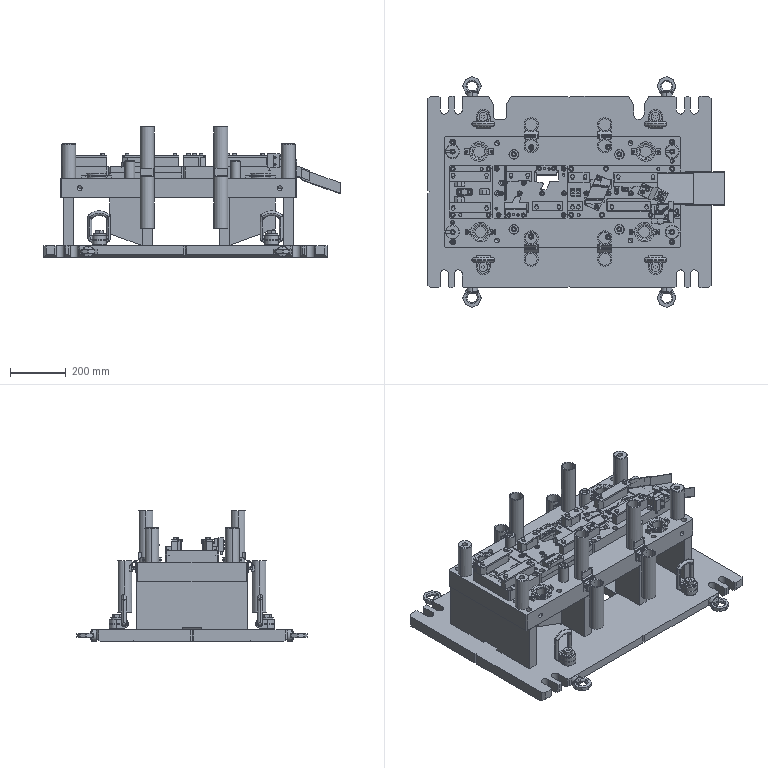Part | CATIA | 151 solids | 4354 faces | volume 67388913 mm3 | cylinder 1701 | plane 1682 | cone 344 | torus 278 | spline 151 | sphere 117 | other 81 | commonest cylinder face diameters 18 x131 10 x129 8 x111 2 x100 6 x94 13 x94